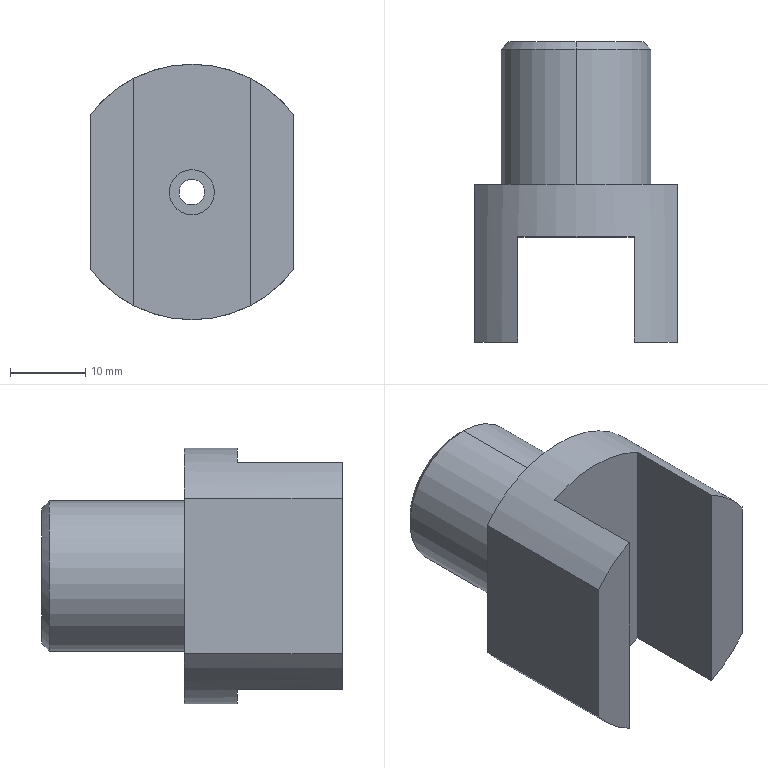Part | STEP file | PN_0016 | 1 solid | 26 faces | box 27 x 40 x 34 mm | volume 14723 mm3 | cylinder 11 | plane 11 | cone 4 | commonest cylinder face diameters 34 x3 3.4 x2 6 x2 8 x2 20 x2